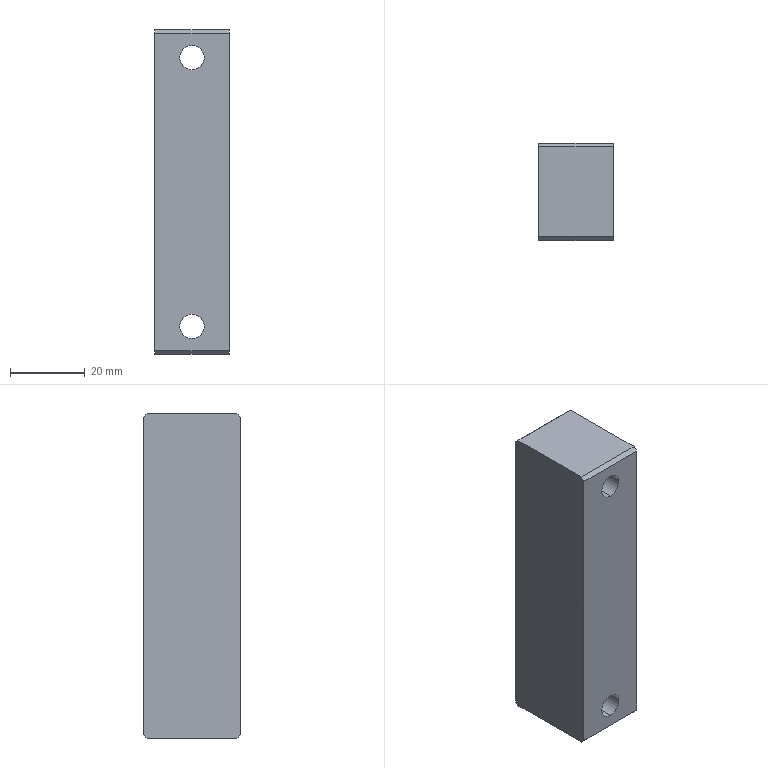Part | STEP file | Riser plate 4_sand-blasted, oxidised | 1 solid | 14 faces | box 20 x 26 x 87 mm | volume 43474 mm3 | plane 10 | cylinder 4 | commonest cylinder face diameters 6.5 x4
STEP:
#1=CARTESIAN_POINT('',(0.,0.,0.));
#2=DIRECTION('',(0.,0.,1.));
#3=DIRECTION('',(1.,0.,0.));
#4=AXIS2_PLACEMENT_3D('',#1,#2,#3);
#5=CARTESIAN_POINT('',(-10.,-13.65,-32.75));
#6=VERTEX_POINT('',#5);
#7=CARTESIAN_POINT('',(-10.,12.35,-32.75));
#8=VERTEX_POINT('',#7);
#9=CARTESIAN_POINT('',(-10.,97.,-32.75));
#10=DIRECTION('',(0.,1.,0.));
#11=VECTOR('',#10,1.);
#12=LINE('',#9,#11);
#13=CARTESIAN_POINT('',(-10.,97.,-36.));
#14=DIRECTION('',(0.,1.,0.));
#15=DIRECTION('',(0.,0.,1.));
#16=AXIS2_PLACEMENT_3D('',#13,#14,#15);
#17=CYLINDRICAL_SURFACE('',#16,3.25);
#18=CARTESIAN_POINT('',(6.283,0.));
#19=DIRECTION('',(0.,1.));
#20=VECTOR('',#19,1.);
#21=LINE('',#18,#20);
#22=(GEOMETRIC_REPRESENTATION_CONTEXT(2)PARAMETRIC_REPRESENTATION_CONTEXT()REPRESENTATION_CONTEXT('',''));
#23=DEFINITIONAL_REPRESENTATION('',(#21),#22);
#24=PCURVE('',#17,#23);
#25=CARTESIAN_POINT('',(-10.,97.,-36.));
#26=DIRECTION('',(0.,1.,0.));
#27=DIRECTION('',(0.,0.,1.));
#28=AXIS2_PLACEMENT_3D('',#25,#26,#27);
#29=CYLINDRICAL_SURFACE('',#28,3.25);
#30=CARTESIAN_POINT('',(0.,0.));
#31=DIRECTION('',(0.,1.));
#32=VECTOR('',#31,1.);
#33=LINE('',#30,#32);
#34=(GEOMETRIC_REPRESENTATION_CONTEXT(2)PARAMETRIC_REPRESENTATION_CONTEXT()REPRESENTATION_CONTEXT('',''));
#35=DEFINITIONAL_REPRESENTATION('',(#33),#34);
#36=PCURVE('',#29,#35);
#37=SURFACE_CURVE('',#12,(#24,#36),.PCURVE_S1.);
#38=EDGE_CURVE('',#6,#8,#37,.T.);
#39=ORIENTED_EDGE('',*,*,#38,.T.);
#40=CARTESIAN_POINT('',(-10.,12.35,-39.25));
#41=VERTEX_POINT('',#40);
#42=CARTESIAN_POINT('',(-10.,12.35,-36.));
#43=DIRECTION('',(0.,-1.,0.));
#44=DIRECTION('',(0.,0.,-1.));
#45=AXIS2_PLACEMENT_3D('',#42,#43,#44);
#46=CIRCLE('',#45,3.25);
#47=CARTESIAN_POINT('',(9.425,-84.65));
#48=DIRECTION('',(-1.,0.));
#49=VECTOR('',#48,1.);
#50=LINE('',#47,#49);
#51=(GEOMETRIC_REPRESENTATION_CONTEXT(2)PARAMETRIC_REPRESENTATION_CONTEXT()REPRESENTATION_CONTEXT('',''));
#52=DEFINITIONAL_REPRESENTATION('',(#50),#51);
#53=PCURVE('',#17,#52);
#54=CARTESIAN_POINT('',(0.,12.35,-43.5));
#55=DIRECTION('',(0.,-1.,0.));
#56=DIRECTION('',(0.,0.,-1.));
#57=AXIS2_PLACEMENT_3D('',#54,#55,#56);
#58=PLANE('',#57);
#59=CARTESIAN_POINT('',(-7.5,-10.));
#60=DIRECTION('',(1.,0.));
#61=AXIS2_PLACEMENT_2D('',#59,#60);
#62=CIRCLE('',#61,3.25);
#63=(GEOMETRIC_REPRESENTATION_CONTEXT(2)PARAMETRIC_REPRESENTATION_CONTEXT()REPRESENTATION_CONTEXT('',''));
#64=DEFINITIONAL_REPRESENTATION('',(#62),#63);
#65=PCURVE('',#58,#64);
#66=SURFACE_CURVE('',#46,(#53,#65),.PCURVE_S1.);
#67=EDGE_CURVE('',#8,#41,#66,.T.);
#68=ORIENTED_EDGE('',*,*,#67,.T.);
#69=CARTESIAN_POINT('',(-10.,-13.65,-39.25));
#70=VERTEX_POINT('',#69);
#71=CARTESIAN_POINT('',(-10.,97.,-39.25));
#72=DIRECTION('',(0.,1.,0.));
#73=VECTOR('',#72,1.);
#74=LINE('',#71,#73);
#75=CARTESIAN_POINT('',(3.142,0.));
#76=DIRECTION('',(0.,1.));
#77=VECTOR('',#76,1.);
#78=LINE('',#75,#77);
#79=(GEOMETRIC_REPRESENTATION_CONTEXT(2)PARAMETRIC_REPRESENTATION_CONTEXT()REPRESENTATION_CONTEXT('',''));
#80=DEFINITIONAL_REPRESENTATION('',(#78),#79);
#81=PCURVE('',#17,#80);
#82=CARTESIAN_POINT('',(3.142,0.));
#83=DIRECTION('',(0.,1.));
#84=VECTOR('',#83,1.);
#85=LINE('',#82,#84);
#86=(GEOMETRIC_REPRESENTATION_CONTEXT(2)PARAMETRIC_REPRESENTATION_CONTEXT()REPRESENTATION_CONTEXT('',''));
#87=DEFINITIONAL_REPRESENTATION('',(#85),#86);
#88=PCURVE('',#29,#87);
#89=SURFACE_CURVE('',#74,(#81,#88),.PCURVE_S1.);
#90=EDGE_CURVE('',#70,#41,#89,.T.);
#91=ORIENTED_EDGE('',*,*,#90,.F.);
#92=CARTESIAN_POINT('',(-10.,-13.65,-36.));
#93=DIRECTION('',(0.,1.,0.));
#94=DIRECTION('',(0.,0.,1.));
#95=AXIS2_PLACEMENT_3D('',#92,#93,#94);
#96=CIRCLE('',#95,3.25);
#97=CARTESIAN_POINT('',(0.,-110.65));
#98=DIRECTION('',(1.,0.));
#99=VECTOR('',#98,1.);
#100=LINE('',#97,#99);
#101=(GEOMETRIC_REPRESENTATION_CONTEXT(2)PARAMETRIC_REPRESENTATION_CONTEXT()REPRESENTATION_CONTEXT('',''));
#102=DEFINITIONAL_REPRESENTATION('',(#100),#101);
#103=PCURVE('',#17,#102);
#104=CARTESIAN_POINT('',(0.,-13.65,43.5));
#105=DIRECTION('',(0.,1.,0.));
#106=DIRECTION('',(-1.,0.,0.));
#107=AXIS2_PLACEMENT_3D('',#104,#105,#106);
#108=PLANE('',#107);
#109=CARTESIAN_POINT('',(10.,-79.5));
#110=DIRECTION('',(0.,1.));
#111=AXIS2_PLACEMENT_2D('',#109,#110);
#112=CIRCLE('',#111,3.25);
#113=(GEOMETRIC_REPRESENTATION_CONTEXT(2)PARAMETRIC_REPRESENTATION_CONTEXT()REPRESENTATION_CONTEXT('',''));
#114=DEFINITIONAL_REPRESENTATION('',(#112),#113);
#115=PCURVE('',#108,#114);
#116=SURFACE_CURVE('',#96,(#103,#115),.PCURVE_S1.);
#117=EDGE_CURVE('',#70,#6,#116,.T.);
#118=ORIENTED_EDGE('',*,*,#117,.T.);
#119=EDGE_LOOP('',(#39,#68,#91,#118));
#120=FACE_BOUND('',#119,.F.);
#121=ADVANCED_FACE('',(#120),#17,.F.);
#122=CARTESIAN_POINT('',(-10.,-13.65,39.25));
#123=VERTEX_POINT('',#122);
#124=CARTESIAN_POINT('',(-10.,12.35,39.25));
#125=VERTEX_POINT('',#124);
#126=CARTESIAN_POINT('',(-10.,97.,39.25));
#127=DIRECTION('',(0.,1.,0.));
#128=VECTOR('',#127,1.);
#129=LINE('',#126,#128);
#130=CARTESIAN_POINT('',(-10.,97.,36.));
#131=DIRECTION('',(0.,1.,0.));
#132=DIRECTION('',(0.,0.,1.));
#133=AXIS2_PLACEMENT_3D('',#130,#131,#132);
#134=CYLINDRICAL_SURFACE('',#133,3.25);
#135=CARTESIAN_POINT('',(6.283,0.));
#136=DIRECTION('',(0.,1.));
#137=VECTOR('',#136,1.);
#138=LINE('',#135,#137);
#139=(GEOMETRIC_REPRESENTATION_CONTEXT(2)PARAMETRIC_REPRESENTATION_CONTEXT()REPRESENTATION_CONTEXT('',''));
#140=DEFINITIONAL_REPRESENTATION('',(#138),#139);
#141=PCURVE('',#134,#140);
#142=CARTESIAN_POINT('',(-10.,97.,36.));
#143=DIRECTION('',(0.,1.,0.));
#144=DIRECTION('',(0.,0.,1.));
#145=AXIS2_PLACEMENT_3D('',#142,#143,#144);
#146=CYLINDRICAL_SURFACE('',#145,3.25);
#147=CARTESIAN_POINT('',(0.,0.));
#148=DIRECTION('',(0.,1.));
#149=VECTOR('',#148,1.);
#150=LINE('',#147,#149);
#151=(GEOMETRIC_REPRESENTATION_CONTEXT(2)PARAMETRIC_REPRESENTATION_CONTEXT()REPRESENTATION_CONTEXT('',''));
#152=DEFINITIONAL_REPRESENTATION('',(#150),#151);
#153=PCURVE('',#146,#152);
#154=SURFACE_CURVE('',#129,(#141,#153),.PCURVE_S1.);
#155=EDGE_CURVE('',#123,#125,#154,.T.);
#156=ORIENTED_EDGE('',*,*,#155,.T.);
#157=CARTESIAN_POINT('',(-10.,12.35,32.75));
#158=VERTEX_POINT('',#157);
#159=CARTESIAN_POINT('',(-10.,12.35,36.));
#160=DIRECTION('',(0.,-1.,0.));
#161=DIRECTION('',(0.,0.,-1.));
#162=AXIS2_PLACEMENT_3D('',#159,#160,#161);
#163=CIRCLE('',#162,3.25);
#164=CARTESIAN_POINT('',(9.425,-84.65));
#165=DIRECTION('',(-1.,0.));
#166=VECTOR('',#165,1.);
#167=LINE('',#164,#166);
#168=(GEOMETRIC_REPRESENTATION_CONTEXT(2)PARAMETRIC_REPRESENTATION_CONTEXT()REPRESENTATION_CONTEXT('',''));
#169=DEFINITIONAL_REPRESENTATION('',(#167),#168);
#170=PCURVE('',#134,#169);
#171=CARTESIAN_POINT('',(-79.5,-10.));
#172=DIRECTION('',(1.,0.));
#173=AXIS2_PLACEMENT_2D('',#171,#172);
#174=CIRCLE('',#173,3.25);
#175=(GEOMETRIC_REPRESENTATION_CONTEXT(2)PARAMETRIC_REPRESENTATION_CONTEXT()REPRESENTATION_CONTEXT('',''));
#176=DEFINITIONAL_REPRESENTATION('',(#174),#175);
#177=PCURVE('',#58,#176);
#178=SURFACE_CURVE('',#163,(#170,#177),.PCURVE_S1.);
#179=EDGE_CURVE('',#125,#158,#178,.T.);
#180=ORIENTED_EDGE('',*,*,#179,.T.);
#181=CARTESIAN_POINT('',(-10.,-13.65,32.75));
#182=VERTEX_POINT('',#181);
#183=CARTESIAN_POINT('',(-10.,97.,32.75));
#184=DIRECTION('',(0.,1.,0.));
#185=VECTOR('',#184,1.);
#186=LINE('',#183,#185);
#187=CARTESIAN_POINT('',(3.142,0.));
#188=DIRECTION('',(0.,1.));
#189=VECTOR('',#188,1.);
#190=LINE('',#187,#189);
#191=(GEOMETRIC_REPRESENTATION_CONTEXT(2)PARAMETRIC_REPRESENTATION_CONTEXT()REPRESENTATION_CONTEXT('',''));
#192=DEFINITIONAL_REPRESENTATION('',(#190),#191);
#193=PCURVE('',#134,#192);
#194=CARTESIAN_POINT('',(3.142,0.));
#195=DIRECTION('',(0.,1.));
#196=VECTOR('',#195,1.);
#197=LINE('',#194,#196);
#198=(GEOMETRIC_REPRESENTATION_CONTEXT(2)PARAMETRIC_REPRESENTATION_CONTEXT()REPRESENTATION_CONTEXT('',''));
#199=DEFINITIONAL_REPRESENTATION('',(#197),#198);
#200=PCURVE('',#146,#199);
#201=SURFACE_CURVE('',#186,(#193,#200),.PCURVE_S1.);
#202=EDGE_CURVE('',#182,#158,#201,.T.);
#203=ORIENTED_EDGE('',*,*,#202,.F.);
#204=CARTESIAN_POINT('',(-10.,-13.65,36.));
#205=DIRECTION('',(0.,1.,0.));
#206=DIRECTION('',(0.,0.,1.));
#207=AXIS2_PLACEMENT_3D('',#204,#205,#206);
#208=CIRCLE('',#207,3.25);
#209=CARTESIAN_POINT('',(0.,-110.65));
#210=DIRECTION('',(1.,0.));
#211=VECTOR('',#210,1.);
#212=LINE('',#209,#211);
#213=(GEOMETRIC_REPRESENTATION_CONTEXT(2)PARAMETRIC_REPRESENTATION_CONTEXT()REPRESENTATION_CONTEXT('',''));
#214=DEFINITIONAL_REPRESENTATION('',(#212),#213);
#215=PCURVE('',#134,#214);
#216=CARTESIAN_POINT('',(10.,-7.5));
#217=DIRECTION('',(0.,1.));
#218=AXIS2_PLACEMENT_2D('',#216,#217);
#219=CIRCLE('',#218,3.25);
#220=(GEOMETRIC_REPRESENTATION_CONTEXT(2)PARAMETRIC_REPRESENTATION_CONTEXT()REPRESENTATION_CONTEXT('',''));
#221=DEFINITIONAL_REPRESENTATION('',(#219),#220);
#222=PCURVE('',#108,#221);
#223=SURFACE_CURVE('',#208,(#215,#222),.PCURVE_S1.);
#224=EDGE_CURVE('',#182,#123,#223,.T.);
#225=ORIENTED_EDGE('',*,*,#224,.T.);
#226=EDGE_LOOP('',(#156,#180,#203,#225));
#227=FACE_BOUND('',#226,.F.);
#228=ADVANCED_FACE('',(#227),#134,.F.);
#229=CARTESIAN_POINT('',(-20.,11.35,43.5));
#230=VERTEX_POINT('',#229);
#231=CARTESIAN_POINT('',(-20.,-12.65,43.5));
#232=VERTEX_POINT('',#231);
#233=CARTESIAN_POINT('',(-20.,0.,43.5));
#234=DIRECTION('',(0.,-1.,0.));
#235=VECTOR('',#234,1.);
#236=LINE('',#233,#235);
#237=CARTESIAN_POINT('',(0.,0.,43.5));
#238=DIRECTION('',(0.,0.,-1.));
#239=DIRECTION('',(-1.,0.,0.));
#240=AXIS2_PLACEMENT_3D('',#237,#238,#239);
#241=PLANE('',#240);
#242=CARTESIAN_POINT('',(20.,0.));
#243=DIRECTION('',(0.,-1.));
#244=VECTOR('',#243,1.);
#245=LINE('',#242,#244);
#246=(GEOMETRIC_REPRESENTATION_CONTEXT(2)PARAMETRIC_REPRESENTATION_CONTEXT()REPRESENTATION_CONTEXT('',''));
#247=DEFINITIONAL_REPRESENTATION('',(#245),#246);
#248=PCURVE('',#241,#247);
#249=CARTESIAN_POINT('',(-20.,0.,43.5));
#250=DIRECTION('',(1.,0.,0.));
#251=DIRECTION('',(0.,0.,-1.));
#252=AXIS2_PLACEMENT_3D('',#249,#250,#251);
#253=PLANE('',#252);
#254=CARTESIAN_POINT('',(0.,0.));
#255=DIRECTION('',(0.,-1.));
#256=VECTOR('',#255,1.);
#257=LINE('',#254,#256);
#258=(GEOMETRIC_REPRESENTATION_CONTEXT(2)PARAMETRIC_REPRESENTATION_CONTEXT()REPRESENTATION_CONTEXT('',''));
#259=DEFINITIONAL_REPRESENTATION('',(#257),#258);
#260=PCURVE('',#253,#259);
#261=SURFACE_CURVE('',#236,(#248,#260),.PCURVE_S1.);
#262=EDGE_CURVE('',#230,#232,#261,.T.);
#263=ORIENTED_EDGE('',*,*,#262,.T.);
#264=CARTESIAN_POINT('',(0.,-12.65,43.5));
#265=VERTEX_POINT('',#264);
#266=CARTESIAN_POINT('',(0.,-12.65,43.5));
#267=DIRECTION('',(1.,0.,0.));
#268=VECTOR('',#267,1.);
#269=LINE('',#266,#268);
#270=CARTESIAN_POINT('',(0.,-12.65));
#271=DIRECTION('',(-1.,0.));
#272=VECTOR('',#271,1.);
#273=LINE('',#270,#272);
#274=(GEOMETRIC_REPRESENTATION_CONTEXT(2)PARAMETRIC_REPRESENTATION_CONTEXT()REPRESENTATION_CONTEXT('',''));
#275=DEFINITIONAL_REPRESENTATION('',(#273),#274);
#276=PCURVE('',#241,#275);
#277=CARTESIAN_POINT('',(0.,-12.65,43.5));
#278=DIRECTION('',(0.,0.7071,-0.7071));
#279=DIRECTION('',(1.,0.,0.));
#280=AXIS2_PLACEMENT_3D('',#277,#278,#279);
#281=PLANE('',#280);
#282=CARTESIAN_POINT('',(0.,0.));
#283=DIRECTION('',(1.,0.));
#284=VECTOR('',#283,1.);
#285=LINE('',#282,#284);
#286=(GEOMETRIC_REPRESENTATION_CONTEXT(2)PARAMETRIC_REPRESENTATION_CONTEXT()REPRESENTATION_CONTEXT('',''));
#287=DEFINITIONAL_REPRESENTATION('',(#285),#286);
#288=PCURVE('',#281,#287);
#289=SURFACE_CURVE('',#269,(#276,#288),.PCURVE_S1.);
#290=EDGE_CURVE('',#232,#265,#289,.T.);
#291=ORIENTED_EDGE('',*,*,#290,.T.);
#292=CARTESIAN_POINT('',(0.,11.35,43.5));
#293=VERTEX_POINT('',#292);
#294=CARTESIAN_POINT('',(0.,97.,43.5));
#295=DIRECTION('',(0.,1.,0.));
#296=VECTOR('',#295,1.);
#297=LINE('',#294,#296);
#298=CARTESIAN_POINT('',(0.,97.));
#299=DIRECTION('',(0.,1.));
#300=VECTOR('',#299,1.);
#301=LINE('',#298,#300);
#302=(GEOMETRIC_REPRESENTATION_CONTEXT(2)PARAMETRIC_REPRESENTATION_CONTEXT()REPRESENTATION_CONTEXT('',''));
#303=DEFINITIONAL_REPRESENTATION('',(#301),#302);
#304=PCURVE('',#241,#303);
#305=CARTESIAN_POINT('',(0.,97.,43.5));
#306=DIRECTION('',(-1.,0.,0.));
#307=DIRECTION('',(0.,-1.,0.));
#308=AXIS2_PLACEMENT_3D('',#305,#306,#307);
#309=PLANE('',#308);
#310=CARTESIAN_POINT('',(0.,0.));
#311=DIRECTION('',(-1.,0.));
#312=VECTOR('',#311,1.);
#313=LINE('',#310,#312);
#314=(GEOMETRIC_REPRESENTATION_CONTEXT(2)PARAMETRIC_REPRESENTATION_CONTEXT()REPRESENTATION_CONTEXT('',''));
#315=DEFINITIONAL_REPRESENTATION('',(#313),#314);
#316=PCURVE('',#309,#315);
#317=SURFACE_CURVE('',#297,(#304,#316),.PCURVE_S1.);
#318=EDGE_CURVE('',#265,#293,#317,.T.);
#319=ORIENTED_EDGE('',*,*,#318,.T.);
#320=CARTESIAN_POINT('',(0.,11.35,43.5));
#321=DIRECTION('',(-1.,0.,0.));
#322=VECTOR('',#321,1.);
#323=LINE('',#320,#322);
#324=CARTESIAN_POINT('',(0.,11.35));
#325=DIRECTION('',(1.,0.));
#326=VECTOR('',#325,1.);
#327=LINE('',#324,#326);
#328=(GEOMETRIC_REPRESENTATION_CONTEXT(2)PARAMETRIC_REPRESENTATION_CONTEXT()REPRESENTATION_CONTEXT('',''));
#329=DEFINITIONAL_REPRESENTATION('',(#327),#328);
#330=PCURVE('',#241,#329);
#331=CARTESIAN_POINT('',(0.,11.35,43.5));
#332=DIRECTION('',(0.,-0.7071,-0.7071));
#333=DIRECTION('',(-1.,0.,0.));
#334=AXIS2_PLACEMENT_3D('',#331,#332,#333);
#335=PLANE('',#334);
#336=CARTESIAN_POINT('',(0.,0.));
#337=DIRECTION('',(1.,0.));
#338=VECTOR('',#337,1.);
#339=LINE('',#336,#338);
#340=(GEOMETRIC_REPRESENTATION_CONTEXT(2)PARAMETRIC_REPRESENTATION_CONTEXT()REPRESENTATION_CONTEXT('',''));
#341=DEFINITIONAL_REPRESENTATION('',(#339),#340);
#342=PCURVE('',#335,#341);
#343=SURFACE_CURVE('',#323,(#330,#342),.PCURVE_S1.);
#344=EDGE_CURVE('',#293,#230,#343,.T.);
#345=ORIENTED_EDGE('',*,*,#344,.T.);
#346=EDGE_LOOP('',(#263,#291,#319,#345));
#347=FACE_BOUND('',#346,.T.);
#348=ADVANCED_FACE('',(#347),#241,.F.);
#349=CARTESIAN_POINT('',(0.,11.35,-43.5));
#350=VERTEX_POINT('',#349);
#351=CARTESIAN_POINT('',(0.,12.35,-42.5));
#352=VERTEX_POINT('',#351);
#353=CARTESIAN_POINT('',(0.,12.35,-42.5));
#354=DIRECTION('',(0.,0.7071,0.7071));
#355=VECTOR('',#354,1.);
#356=LINE('',#353,#355);
#357=CARTESIAN_POINT('',(84.65,-86.));
#358=DIRECTION('',(-0.7071,0.7071));
#359=VECTOR('',#358,1.);
#360=LINE('',#357,#359);
#361=(GEOMETRIC_REPRESENTATION_CONTEXT(2)PARAMETRIC_REPRESENTATION_CONTEXT()REPRESENTATION_CONTEXT('',''));
#362=DEFINITIONAL_REPRESENTATION('',(#360),#361);
#363=PCURVE('',#309,#362);
#364=CARTESIAN_POINT('',(0.,12.35,-42.5));
#365=DIRECTION('',(0.,0.7071,-0.7071));
#366=DIRECTION('',(1.,0.,0.));
#367=AXIS2_PLACEMENT_3D('',#364,#365,#366);
#368=PLANE('',#367);
#369=CARTESIAN_POINT('',(0.,0.));
#370=DIRECTION('',(0.,-1.));
#371=VECTOR('',#370,1.);
#372=LINE('',#369,#371);
#373=(GEOMETRIC_REPRESENTATION_CONTEXT(2)PARAMETRIC_REPRESENTATION_CONTEXT()REPRESENTATION_CONTEXT('',''));
#374=DEFINITIONAL_REPRESENTATION('',(#372),#373);
#375=PCURVE('',#368,#374);
#376=SURFACE_CURVE('',#356,(#363,#375),.PCURVE_S1.);
#377=EDGE_CURVE('',#350,#352,#376,.T.);
#378=ORIENTED_EDGE('',*,*,#377,.T.);
#379=CARTESIAN_POINT('',(0.,12.35,42.5));
#380=VERTEX_POINT('',#379);
#381=CARTESIAN_POINT('',(0.,12.35,43.5));
#382=DIRECTION('',(0.,0.,1.));
#383=VECTOR('',#382,1.);
#384=LINE('',#381,#383);
#385=CARTESIAN_POINT('',(84.65,0.));
#386=DIRECTION('',(0.,1.));
#387=VECTOR('',#386,1.);
#388=LINE('',#385,#387);
#389=(GEOMETRIC_REPRESENTATION_CONTEXT(2)PARAMETRIC_REPRESENTATION_CONTEXT()REPRESENTATION_CONTEXT('',''));
#390=DEFINITIONAL_REPRESENTATION('',(#388),#389);
#391=PCURVE('',#309,#390);
#392=CARTESIAN_POINT('',(-87.,0.));
#393=DIRECTION('',(-1.,0.));
#394=VECTOR('',#393,1.);
#395=LINE('',#392,#394);
#396=(GEOMETRIC_REPRESENTATION_CONTEXT(2)PARAMETRIC_REPRESENTATION_CONTEXT()REPRESENTATION_CONTEXT('',''));
#397=DEFINITIONAL_REPRESENTATION('',(#395),#396);
#398=PCURVE('',#58,#397);
#399=SURFACE_CURVE('',#384,(#391,#398),.PCURVE_S1.);
#400=EDGE_CURVE('',#352,#380,#399,.T.);
#401=ORIENTED_EDGE('',*,*,#400,.T.);
#402=CARTESIAN_POINT('',(0.,11.35,43.5));
#403=DIRECTION('',(0.,-0.7071,0.7071));
#404=VECTOR('',#403,1.);
#405=LINE('',#402,#404);
#406=CARTESIAN_POINT('',(85.65,0.));
#407=DIRECTION('',(0.7071,0.7071));
#408=VECTOR('',#407,1.);
#409=LINE('',#406,#408);
#410=(GEOMETRIC_REPRESENTATION_CONTEXT(2)PARAMETRIC_REPRESENTATION_CONTEXT()REPRESENTATION_CONTEXT('',''));
#411=DEFINITIONAL_REPRESENTATION('',(#409),#410);
#412=PCURVE('',#309,#411);
#413=CARTESIAN_POINT('',(0.,0.));
#414=DIRECTION('',(0.,-1.));
#415=VECTOR('',#414,1.);
#416=LINE('',#413,#415);
#417=(GEOMETRIC_REPRESENTATION_CONTEXT(2)PARAMETRIC_REPRESENTATION_CONTEXT()REPRESENTATION_CONTEXT('',''));
#418=DEFINITIONAL_REPRESENTATION('',(#416),#417);
#419=PCURVE('',#335,#418);
#420=SURFACE_CURVE('',#405,(#412,#419),.PCURVE_S1.);
#421=EDGE_CURVE('',#380,#293,#420,.T.);
#422=ORIENTED_EDGE('',*,*,#421,.T.);
#423=ORIENTED_EDGE('',*,*,#318,.F.);
#424=CARTESIAN_POINT('',(0.,-13.65,42.5));
#425=VERTEX_POINT('',#424);
#426=CARTESIAN_POINT('',(0.,-12.65,43.5));
#427=DIRECTION('',(0.,-0.7071,-0.7071));
#428=VECTOR('',#427,1.);
#429=LINE('',#426,#428);
#430=CARTESIAN_POINT('',(109.65,0.));
#431=DIRECTION('',(0.7071,-0.7071));
#432=VECTOR('',#431,1.);
#433=LINE('',#430,#432);
#434=(GEOMETRIC_REPRESENTATION_CONTEXT(2)PARAMETRIC_REPRESENTATION_CONTEXT()REPRESENTATION_CONTEXT('',''));
#435=DEFINITIONAL_REPRESENTATION('',(#433),#434);
#436=PCURVE('',#309,#435);
#437=CARTESIAN_POINT('',(0.,0.));
#438=DIRECTION('',(0.,1.));
#439=VECTOR('',#438,1.);
#440=LINE('',#437,#439);
#441=(GEOMETRIC_REPRESENTATION_CONTEXT(2)PARAMETRIC_REPRESENTATION_CONTEXT()REPRESENTATION_CONTEXT('',''));
#442=DEFINITIONAL_REPRESENTATION('',(#440),#441);
#443=PCURVE('',#281,#442);
#444=SURFACE_CURVE('',#429,(#436,#443),.PCURVE_S1.);
#445=EDGE_CURVE('',#265,#425,#444,.T.);
#446=ORIENTED_EDGE('',*,*,#445,.T.);
#447=CARTESIAN_POINT('',(0.,-13.65,-42.5));
#448=VERTEX_POINT('',#447);
#449=CARTESIAN_POINT('',(0.,-13.65,43.5));
#450=DIRECTION('',(0.,0.,-1.));
#451=VECTOR('',#450,1.);
#452=LINE('',#449,#451);
#453=CARTESIAN_POINT('',(110.65,0.));
#454=DIRECTION('',(0.,-1.));
#455=VECTOR('',#454,1.);
#456=LINE('',#453,#455);
#457=(GEOMETRIC_REPRESENTATION_CONTEXT(2)PARAMETRIC_REPRESENTATION_CONTEXT()REPRESENTATION_CONTEXT('',''));
#458=DEFINITIONAL_REPRESENTATION('',(#456),#457);
#459=PCURVE('',#309,#458);
#460=CARTESIAN_POINT('',(0.,0.));
#461=DIRECTION('',(0.,-1.));
#462=VECTOR('',#461,1.);
#463=LINE('',#460,#462);
#464=(GEOMETRIC_REPRESENTATION_CONTEXT(2)PARAMETRIC_REPRESENTATION_CONTEXT()REPRESENTATION_CONTEXT('',''));
#465=DEFINITIONAL_REPRESENTATION('',(#463),#464);
#466=PCURVE('',#108,#465);
#467=SURFACE_CURVE('',#452,(#459,#466),.PCURVE_S1.);
#468=EDGE_CURVE('',#425,#448,#467,.T.);
#469=ORIENTED_EDGE('',*,*,#468,.T.);
#470=CARTESIAN_POINT('',(0.,-12.65,-43.5));
#471=VERTEX_POINT('',#470);
#472=CARTESIAN_POINT('',(0.,-13.65,-42.5));
#473=DIRECTION('',(0.,0.7071,-0.7071));
#474=VECTOR('',#473,1.);
#475=LINE('',#472,#474);
#476=CARTESIAN_POINT('',(110.65,-86.));
#477=DIRECTION('',(-0.7071,-0.7071));
#478=VECTOR('',#477,1.);
#479=LINE('',#476,#478);
#480=(GEOMETRIC_REPRESENTATION_CONTEXT(2)PARAMETRIC_REPRESENTATION_CONTEXT()REPRESENTATION_CONTEXT('',''));
#481=DEFINITIONAL_REPRESENTATION('',(#479),#480);
#482=PCURVE('',#309,#481);
#483=CARTESIAN_POINT('',(0.,-13.65,-42.5));
#484=DIRECTION('',(0.,-0.7071,-0.7071));
#485=DIRECTION('',(-1.,0.,0.));
#486=AXIS2_PLACEMENT_3D('',#483,#484,#485);
#487=PLANE('',#486);
#488=CARTESIAN_POINT('',(0.,0.));
#489=DIRECTION('',(0.,1.));
#490=VECTOR('',#489,1.);
#491=LINE('',#488,#490);
#492=(GEOMETRIC_REPRESENTATION_CONTEXT(2)PARAMETRIC_REPRESENTATION_CONTEXT()REPRESENTATION_CONTEXT('',''));
#493=DEFINITIONAL_REPRESENTATION('',(#491),#492);
#494=PCURVE('',#487,#493);
#495=SURFACE_CURVE('',#475,(#482,#494),.PCURVE_S1.);
#496=EDGE_CURVE('',#448,#471,#495,.T.);
#497=ORIENTED_EDGE('',*,*,#496,.T.);
#498=CARTESIAN_POINT('',(0.,97.,-43.5));
#499=DIRECTION('',(0.,1.,0.));
#500=VECTOR('',#499,1.);
#501=LINE('',#498,#500);
#502=CARTESIAN_POINT('',(0.,-87.));
#503=DIRECTION('',(-1.,0.));
#504=VECTOR('',#503,1.);
#505=LINE('',#502,#504);
#506=(GEOMETRIC_REPRESENTATION_CONTEXT(2)PARAMETRIC_REPRESENTATION_CONTEXT()REPRESENTATION_CONTEXT('',''));
#507=DEFINITIONAL_REPRESENTATION('',(#505),#506);
#508=PCURVE('',#309,#507);
#509=CARTESIAN_POINT('',(0.,0.,-43.5));
#510=DIRECTION('',(0.,0.,-1.));
#511=DIRECTION('',(-1.,0.,0.));
#512=AXIS2_PLACEMENT_3D('',#509,#510,#511);
#513=PLANE('',#512);
#514=CARTESIAN_POINT('',(0.,97.));
#515=DIRECTION('',(0.,1.));
#516=VECTOR('',#515,1.);
#517=LINE('',#514,#516);
#518=(GEOMETRIC_REPRESENTATION_CONTEXT(2)PARAMETRIC_REPRESENTATION_CONTEXT()REPRESENTATION_CONTEXT('',''));
#519=DEFINITIONAL_REPRESENTATION('',(#517),#518);
#520=PCURVE('',#513,#519);
#521=SURFACE_CURVE('',#501,(#508,#520),.PCURVE_S1.);
#522=EDGE_CURVE('',#471,#350,#521,.T.);
#523=ORIENTED_EDGE('',*,*,#522,.T.);
#524=EDGE_LOOP('',(#378,#401,#422,#423,#446,#469,#497,#523));
#525=FACE_BOUND('',#524,.T.);
#526=ADVANCED_FACE('',(#525),#309,.F.);
#527=CARTESIAN_POINT('',(-20.,12.35,-42.5));
#528=VERTEX_POINT('',#527);
#529=CARTESIAN_POINT('',(-20.,12.35,42.5));
#530=VERTEX_POINT('',#529);
#531=CARTESIAN_POINT('',(-20.,12.35,43.5));
#532=DIRECTION('',(0.,0.,1.));
#533=VECTOR('',#532,1.);
#534=LINE('',#531,#533);
#535=CARTESIAN_POINT('',(0.,12.35));
#536=DIRECTION('',(-1.,0.));
#537=VECTOR('',#536,1.);
#538=LINE('',#535,#537);
#539=(GEOMETRIC_REPRESENTATION_CONTEXT(2)PARAMETRIC_REPRESENTATION_CONTEXT()REPRESENTATION_CONTEXT('',''));
#540=DEFINITIONAL_REPRESENTATION('',(#538),#539);
#541=PCURVE('',#253,#540);
#542=CARTESIAN_POINT('',(-87.,-20.));
#543=DIRECTION('',(-1.,0.));
#544=VECTOR('',#543,1.);
#545=LINE('',#542,#544);
#546=(GEOMETRIC_REPRESENTATION_CONTEXT(2)PARAMETRIC_REPRESENTATION_CONTEXT()REPRESENTATION_CONTEXT('',''));
#547=DEFINITIONAL_REPRESENTATION('',(#545),#546);
#548=PCURVE('',#58,#547);
#549=SURFACE_CURVE('',#534,(#541,#548),.PCURVE_S1.);
#550=EDGE_CURVE('',#528,#530,#549,.T.);
#551=ORIENTED_EDGE('',*,*,#550,.F.);
#552=CARTESIAN_POINT('',(-20.,11.35,-43.5));
#553=VERTEX_POINT('',#552);
#554=CARTESIAN_POINT('',(-20.,12.35,-42.5));
#555=DIRECTION('',(0.,-0.7071,-0.7071));
#556=VECTOR('',#555,1.);
#557=LINE('',#554,#556);
#558=CARTESIAN_POINT('',(86.,12.35));
#559=DIRECTION('',(0.7071,-0.7071));
#560=VECTOR('',#559,1.);
#561=LINE('',#558,#560);
#562=(GEOMETRIC_REPRESENTATION_CONTEXT(2)PARAMETRIC_REPRESENTATION_CONTEXT()REPRESENTATION_CONTEXT('',''));
#563=DEFINITIONAL_REPRESENTATION('',(#561),#562);
#564=PCURVE('',#253,#563);
#565=CARTESIAN_POINT('',(-20.,0.));
#566=DIRECTION('',(0.,1.));
#567=VECTOR('',#566,1.);
#568=LINE('',#565,#567);
#569=(GEOMETRIC_REPRESENTATION_CONTEXT(2)PARAMETRIC_REPRESENTATION_CONTEXT()REPRESENTATION_CONTEXT('',''));
#570=DEFINITIONAL_REPRESENTATION('',(#568),#569);
#571=PCURVE('',#368,#570);
#572=SURFACE_CURVE('',#557,(#564,#571),.PCURVE_S1.);
#573=EDGE_CURVE('',#528,#553,#572,.T.);
#574=ORIENTED_EDGE('',*,*,#573,.T.);
#575=CARTESIAN_POINT('',(-20.,-12.65,-43.5));
#576=VERTEX_POINT('',#575);
#577=CARTESIAN_POINT('',(-20.,0.,-43.5));
#578=DIRECTION('',(0.,-1.,0.));
#579=VECTOR('',#578,1.);
#580=LINE('',#577,#579);
#581=CARTESIAN_POINT('',(87.,0.));
#582=DIRECTION('',(0.,-1.));
#583=VECTOR('',#582,1.);
#584=LINE('',#581,#583);
#585=(GEOMETRIC_REPRESENTATION_CONTEXT(2)PARAMETRIC_REPRESENTATION_CONTEXT()REPRESENTATION_CONTEXT('',''));
#586=DEFINITIONAL_REPRESENTATION('',(#584),#585);
#587=PCURVE('',#253,#586);
#588=CARTESIAN_POINT('',(20.,0.));
#589=DIRECTION('',(0.,-1.));
#590=VECTOR('',#589,1.);
#591=LINE('',#588,#590);
#592=(GEOMETRIC_REPRESENTATION_CONTEXT(2)PARAMETRIC_REPRESENTATION_CONTEXT()REPRESENTATION_CONTEXT('',''));
#593=DEFINITIONAL_REPRESENTATION('',(#591),#592);
#594=PCURVE('',#513,#593);
#595=SURFACE_CURVE('',#580,(#587,#594),.PCURVE_S1.);
#596=EDGE_CURVE('',#553,#576,#595,.T.);
#597=ORIENTED_EDGE('',*,*,#596,.T.);
#598=CARTESIAN_POINT('',(-20.,-13.65,-42.5));
#599=VERTEX_POINT('',#598);
#600=CARTESIAN_POINT('',(-20.,-13.65,-42.5));
#601=DIRECTION('',(0.,-0.7071,0.7071));
#602=VECTOR('',#601,1.);
#603=LINE('',#600,#602);
#604=CARTESIAN_POINT('',(86.,-13.65));
#605=DIRECTION('',(-0.7071,-0.7071));
#606=VECTOR('',#605,1.);
#607=LINE('',#604,#606);
#608=(GEOMETRIC_REPRESENTATION_CONTEXT(2)PARAMETRIC_REPRESENTATION_CONTEXT()REPRESENTATION_CONTEXT('',''));
#609=DEFINITIONAL_REPRESENTATION('',(#607),#608);
#610=PCURVE('',#253,#609);
#611=CARTESIAN_POINT('',(20.,0.));
#612=DIRECTION('',(0.,-1.));
#613=VECTOR('',#612,1.);
#614=LINE('',#611,#613);
#615=(GEOMETRIC_REPRESENTATION_CONTEXT(2)PARAMETRIC_REPRESENTATION_CONTEXT()REPRESENTATION_CONTEXT('',''));
#616=DEFINITIONAL_REPRESENTATION('',(#614),#615);
#617=PCURVE('',#487,#616);
#618=SURFACE_CURVE('',#603,(#610,#617),.PCURVE_S1.);
#619=EDGE_CURVE('',#576,#599,#618,.T.);
#620=ORIENTED_EDGE('',*,*,#619,.T.);
#621=CARTESIAN_POINT('',(-20.,-13.65,42.5));
#622=VERTEX_POINT('',#621);
#623=CARTESIAN_POINT('',(-20.,-13.65,43.5));
#624=DIRECTION('',(0.,0.,-1.));
#625=VECTOR('',#624,1.);
#626=LINE('',#623,#625);
#627=CARTESIAN_POINT('',(0.,-13.65));
#628=DIRECTION('',(1.,0.));
#629=VECTOR('',#628,1.);
#630=LINE('',#627,#629);
#631=(GEOMETRIC_REPRESENTATION_CONTEXT(2)PARAMETRIC_REPRESENTATION_CONTEXT()REPRESENTATION_CONTEXT('',''));
#632=DEFINITIONAL_REPRESENTATION('',(#630),#631);
#633=PCURVE('',#253,#632);
#634=CARTESIAN_POINT('',(20.,0.));
#635=DIRECTION('',(0.,-1.));
#636=VECTOR('',#635,1.);
#637=LINE('',#634,#636);
#638=(GEOMETRIC_REPRESENTATION_CONTEXT(2)PARAMETRIC_REPRESENTATION_CONTEXT()REPRESENTATION_CONTEXT('',''));
#639=DEFINITIONAL_REPRESENTATION('',(#637),#638);
#640=PCURVE('',#108,#639);
#641=SURFACE_CURVE('',#626,(#633,#640),.PCURVE_S1.);
#642=EDGE_CURVE('',#622,#599,#641,.T.);
#643=ORIENTED_EDGE('',*,*,#642,.F.);
#644=CARTESIAN_POINT('',(-20.,-12.65,43.5));
#645=DIRECTION('',(0.,0.7071,0.7071));
#646=VECTOR('',#645,1.);
#647=LINE('',#644,#646);
#648=CARTESIAN_POINT('',(0.,-12.65));
#649=DIRECTION('',(-0.7071,0.7071));
#650=VECTOR('',#649,1.);
#651=LINE('',#648,#650);
#652=(GEOMETRIC_REPRESENTATION_CONTEXT(2)PARAMETRIC_REPRESENTATION_CONTEXT()REPRESENTATION_CONTEXT('',''));
#653=DEFINITIONAL_REPRESENTATION('',(#651),#652);
#654=PCURVE('',#253,#653);
#655=CARTESIAN_POINT('',(-20.,0.));
#656=DIRECTION('',(0.,-1.));
#657=VECTOR('',#656,1.);
#658=LINE('',#655,#657);
#659=(GEOMETRIC_REPRESENTATION_CONTEXT(2)PARAMETRIC_REPRESENTATION_CONTEXT()REPRESENTATION_CONTEXT('',''));
#660=DEFINITIONAL_REPRESENTATION('',(#658),#659);
#661=PCURVE('',#281,#660);
#662=SURFACE_CURVE('',#647,(#654,#661),.PCURVE_S1.);
#663=EDGE_CURVE('',#622,#232,#662,.T.);
#664=ORIENTED_EDGE('',*,*,#663,.T.);
#665=ORIENTED_EDGE('',*,*,#262,.F.);
#666=CARTESIAN_POINT('',(-20.,11.35,43.5));
#667=DIRECTION('',(0.,0.7071,-0.7071));
#668=VECTOR('',#667,1.);
#669=LINE('',#666,#668);
#670=CARTESIAN_POINT('',(0.,11.35));
#671=DIRECTION('',(0.7071,0.7071));
#672=VECTOR('',#671,1.);
#673=LINE('',#670,#672);
#674=(GEOMETRIC_REPRESENTATION_CONTEXT(2)PARAMETRIC_REPRESENTATION_CONTEXT()REPRESENTATION_CONTEXT('',''));
#675=DEFINITIONAL_REPRESENTATION('',(#673),#674);
#676=PCURVE('',#253,#675);
#677=CARTESIAN_POINT('',(20.,0.));
#678=DIRECTION('',(0.,1.));
#679=VECTOR('',#678,1.);
#680=LINE('',#677,#679);
#681=(GEOMETRIC_REPRESENTATION_CONTEXT(2)PARAMETRIC_REPRESENTATION_CONTEXT()REPRESENTATION_CONTEXT('',''));
#682=DEFINITIONAL_REPRESENTATION('',(#680),#681);
#683=PCURVE('',#335,#682);
#684=SURFACE_CURVE('',#669,(#676,#683),.PCURVE_S1.);
#685=EDGE_CURVE('',#230,#530,#684,.T.);
#686=ORIENTED_EDGE('',*,*,#685,.T.);
#687=EDGE_LOOP('',(#551,#574,#597,#620,#643,#664,#665,#686));
#688=FACE_BOUND('',#687,.T.);
#689=ADVANCED_FACE('',(#688),#253,.F.);
#690=CARTESIAN_POINT('',(-10.,-13.65,-36.));
#691=DIRECTION('',(0.,1.,0.));
#692=DIRECTION('',(0.,0.,1.));
#693=AXIS2_PLACEMENT_3D('',#690,#691,#692);
#694=CIRCLE('',#693,3.25);
#695=CARTESIAN_POINT('',(10.,-79.5));
#696=DIRECTION('',(0.,1.));
#697=AXIS2_PLACEMENT_2D('',#695,#696);
#698=CIRCLE('',#697,3.25);
#699=(GEOMETRIC_REPRESENTATION_CONTEXT(2)PARAMETRIC_REPRESENTATION_CONTEXT()REPRESENTATION_CONTEXT('',''));
#700=DEFINITIONAL_REPRESENTATION('',(#698),#699);
#701=PCURVE('',#108,#700);
#702=CARTESIAN_POINT('',(0.,-110.65));
#703=DIRECTION('',(1.,0.));
#704=VECTOR('',#703,1.);
#705=LINE('',#702,#704);
#706=(GEOMETRIC_REPRESENTATION_CONTEXT(2)PARAMETRIC_REPRESENTATION_CONTEXT()REPRESENTATION_CONTEXT('',''));
#707=DEFINITIONAL_REPRESENTATION('',(#705),#706);
#708=PCURVE('',#29,#707);
#709=SURFACE_CURVE('',#694,(#701,#708),.PCURVE_S1.);
#710=EDGE_CURVE('',#6,#70,#709,.T.);
#711=ORIENTED_EDGE('',*,*,#710,.T.);
#712=ORIENTED_EDGE('',*,*,#117,.T.);
#713=EDGE_LOOP('',(#711,#712));
#714=FACE_BOUND('',#713,.T.);
#715=CARTESIAN_POINT('',(-10.,-13.65,36.));
#716=DIRECTION('',(0.,1.,0.));
#717=DIRECTION('',(0.,0.,1.));
#718=AXIS2_PLACEMENT_3D('',#715,#716,#717);
#719=CIRCLE('',#718,3.25);
#720=CARTESIAN_POINT('',(10.,-7.5));
#721=DIRECTION('',(0.,1.));
#722=AXIS2_PLACEMENT_2D('',#720,#721);
#723=CIRCLE('',#722,3.25);
#724=(GEOMETRIC_REPRESENTATION_CONTEXT(2)PARAMETRIC_REPRESENTATION_CONTEXT()REPRESENTATION_CONTEXT('',''));
#725=DEFINITIONAL_REPRESENTATION('',(#723),#724);
#726=PCURVE('',#108,#725);
#727=CARTESIAN_POINT('',(0.,-110.65));
#728=DIRECTION('',(1.,0.));
#729=VECTOR('',#728,1.);
#730=LINE('',#727,#729);
#731=(GEOMETRIC_REPRESENTATION_CONTEXT(2)PARAMETRIC_REPRESENTATION_CONTEXT()REPRESENTATION_CONTEXT('',''));
#732=DEFINITIONAL_REPRESENTATION('',(#730),#731);
#733=PCURVE('',#146,#732);
#734=SURFACE_CURVE('',#719,(#726,#733),.PCURVE_S1.);
#735=EDGE_CURVE('',#123,#182,#734,.T.);
#736=ORIENTED_EDGE('',*,*,#735,.T.);
#737=ORIENTED_EDGE('',*,*,#224,.T.);
#738=EDGE_LOOP('',(#736,#737));
#739=FACE_BOUND('',#738,.T.);
#740=ORIENTED_EDGE('',*,*,#468,.F.);
#741=CARTESIAN_POINT('',(0.,-13.65,42.5));
#742=DIRECTION('',(-1.,0.,0.));
#743=VECTOR('',#742,1.);
#744=LINE('',#741,#743);
#745=CARTESIAN_POINT('',(0.,-1.));
#746=DIRECTION('',(1.,0.));
#747=VECTOR('',#746,1.);
#748=LINE('',#745,#747);
#749=(GEOMETRIC_REPRESENTATION_CONTEXT(2)PARAMETRIC_REPRESENTATION_CONTEXT()REPRESENTATION_CONTEXT('',''));
#750=DEFINITIONAL_REPRESENTATION('',(#748),#749);
#751=PCURVE('',#108,#750);
#752=CARTESIAN_POINT('',(0.,1.414));
#753=DIRECTION('',(-1.,0.));
#754=VECTOR('',#753,1.);
#755=LINE('',#752,#754);
#756=(GEOMETRIC_REPRESENTATION_CONTEXT(2)PARAMETRIC_REPRESENTATION_CONTEXT()REPRESENTATION_CONTEXT('',''));
#757=DEFINITIONAL_REPRESENTATION('',(#755),#756);
#758=PCURVE('',#281,#757);
#759=SURFACE_CURVE('',#744,(#751,#758),.PCURVE_S1.);
#760=EDGE_CURVE('',#425,#622,#759,.T.);
#761=ORIENTED_EDGE('',*,*,#760,.T.);
#762=ORIENTED_EDGE('',*,*,#642,.T.);
#763=CARTESIAN_POINT('',(0.,-13.65,-42.5));
#764=DIRECTION('',(1.,0.,0.));
#765=VECTOR('',#764,1.);
#766=LINE('',#763,#765);
#767=CARTESIAN_POINT('',(0.,-86.));
#768=DIRECTION('',(-1.,0.));
#769=VECTOR('',#768,1.);
#770=LINE('',#767,#769);
#771=(GEOMETRIC_REPRESENTATION_CONTEXT(2)PARAMETRIC_REPRESENTATION_CONTEXT()REPRESENTATION_CONTEXT('',''));
#772=DEFINITIONAL_REPRESENTATION('',(#770),#771);
#773=PCURVE('',#108,#772);
#774=CARTESIAN_POINT('',(0.,0.));
#775=DIRECTION('',(-1.,0.));
#776=VECTOR('',#775,1.);
#777=LINE('',#774,#776);
#778=(GEOMETRIC_REPRESENTATION_CONTEXT(2)PARAMETRIC_REPRESENTATION_CONTEXT()REPRESENTATION_CONTEXT('',''));
#779=DEFINITIONAL_REPRESENTATION('',(#777),#778);
#780=PCURVE('',#487,#779);
#781=SURFACE_CURVE('',#766,(#773,#780),.PCURVE_S1.);
#782=EDGE_CURVE('',#599,#448,#781,.T.);
#783=ORIENTED_EDGE('',*,*,#782,.T.);
#784=EDGE_LOOP('',(#740,#761,#762,#783));
#785=FACE_BOUND('',#784,.T.);
#786=ADVANCED_FACE('',(#714,#739,#785),#108,.F.);
#787=ORIENTED_EDGE('',*,*,#522,.F.);
#788=CARTESIAN_POINT('',(-20.,-12.65,-43.5));
#789=DIRECTION('',(-1.,0.,0.));
#790=VECTOR('',#789,1.);
#791=LINE('',#788,#790);
#792=CARTESIAN_POINT('',(20.,-12.65));
#793=DIRECTION('',(1.,0.));
#794=VECTOR('',#793,1.);
#795=LINE('',#792,#794);
#796=(GEOMETRIC_REPRESENTATION_CONTEXT(2)PARAMETRIC_REPRESENTATION_CONTEXT()REPRESENTATION_CONTEXT('',''));
#797=DEFINITIONAL_REPRESENTATION('',(#795),#796);
#798=PCURVE('',#513,#797);
#799=CARTESIAN_POINT('',(20.,1.414));
#800=DIRECTION('',(1.,0.));
#801=VECTOR('',#800,1.);
#802=LINE('',#799,#801);
#803=(GEOMETRIC_REPRESENTATION_CONTEXT(2)PARAMETRIC_REPRESENTATION_CONTEXT()REPRESENTATION_CONTEXT('',''));
#804=DEFINITIONAL_REPRESENTATION('',(#802),#803);
#805=PCURVE('',#487,#804);
#806=SURFACE_CURVE('',#791,(#798,#805),.PCURVE_S1.);
#807=EDGE_CURVE('',#471,#576,#806,.T.);
#808=ORIENTED_EDGE('',*,*,#807,.T.);
#809=ORIENTED_EDGE('',*,*,#596,.F.);
#810=CARTESIAN_POINT('',(0.,11.35,-43.5));
#811=DIRECTION('',(1.,0.,0.));
#812=VECTOR('',#811,1.);
#813=LINE('',#810,#812);
#814=CARTESIAN_POINT('',(0.,11.35));
#815=DIRECTION('',(-1.,0.));
#816=VECTOR('',#815,1.);
#817=LINE('',#814,#816);
#818=(GEOMETRIC_REPRESENTATION_CONTEXT(2)PARAMETRIC_REPRESENTATION_CONTEXT()REPRESENTATION_CONTEXT('',''));
#819=DEFINITIONAL_REPRESENTATION('',(#817),#818);
#820=PCURVE('',#513,#819);
#821=CARTESIAN_POINT('',(0.,1.414));
#822=DIRECTION('',(1.,0.));
#823=VECTOR('',#822,1.);
#824=LINE('',#821,#823);
#825=(GEOMETRIC_REPRESENTATION_CONTEXT(2)PARAMETRIC_REPRESENTATION_CONTEXT()REPRESENTATION_CONTEXT('',''));
#826=DEFINITIONAL_REPRESENTATION('',(#824),#825);
#827=PCURVE('',#368,#826);
#828=SURFACE_CURVE('',#813,(#820,#827),.PCURVE_S1.);
#829=EDGE_CURVE('',#553,#350,#828,.T.);
#830=ORIENTED_EDGE('',*,*,#829,.T.);
#831=EDGE_LOOP('',(#787,#808,#809,#830));
#832=FACE_BOUND('',#831,.T.);
#833=ADVANCED_FACE('',(#832),#513,.T.);
#834=ORIENTED_EDGE('',*,*,#67,.T.);
#835=CARTESIAN_POINT('',(-10.,12.35,-36.));
#836=DIRECTION('',(0.,-1.,0.));
#837=DIRECTION('',(0.,0.,-1.));
#838=AXIS2_PLACEMENT_3D('',#835,#836,#837);
#839=CIRCLE('',#838,3.25);
#840=CARTESIAN_POINT('',(-7.5,-10.));
#841=DIRECTION('',(1.,0.));
#842=AXIS2_PLACEMENT_2D('',#840,#841);
#843=CIRCLE('',#842,3.25);
#844=(GEOMETRIC_REPRESENTATION_CONTEXT(2)PARAMETRIC_REPRESENTATION_CONTEXT()REPRESENTATION_CONTEXT('',''));
#845=DEFINITIONAL_REPRESENTATION('',(#843),#844);
#846=PCURVE('',#58,#845);
#847=CARTESIAN_POINT('',(3.142,-84.65));
#848=DIRECTION('',(-1.,0.));
#849=VECTOR('',#848,1.);
#850=LINE('',#847,#849);
#851=(GEOMETRIC_REPRESENTATION_CONTEXT(2)PARAMETRIC_REPRESENTATION_CONTEXT()REPRESENTATION_CONTEXT('',''));
#852=DEFINITIONAL_REPRESENTATION('',(#850),#851);
#853=PCURVE('',#29,#852);
#854=SURFACE_CURVE('',#839,(#846,#853),.PCURVE_S1.);
#855=EDGE_CURVE('',#41,#8,#854,.T.);
#856=ORIENTED_EDGE('',*,*,#855,.T.);
#857=EDGE_LOOP('',(#834,#856));
#858=FACE_BOUND('',#857,.T.);
#859=ORIENTED_EDGE('',*,*,#400,.F.);
#860=CARTESIAN_POINT('',(-20.,12.35,-42.5));
#861=DIRECTION('',(-1.,0.,0.));
#862=VECTOR('',#861,1.);
#863=LINE('',#860,#862);
#864=CARTESIAN_POINT('',(-1.,-20.));
#865=DIRECTION('',(0.,-1.));
#866=VECTOR('',#865,1.);
#867=LINE('',#864,#866);
#868=(GEOMETRIC_REPRESENTATION_CONTEXT(2)PARAMETRIC_REPRESENTATION_CONTEXT()REPRESENTATION_CONTEXT('',''));
#869=DEFINITIONAL_REPRESENTATION('',(#867),#868);
#870=PCURVE('',#58,#869);
#871=CARTESIAN_POINT('',(-20.,0.));
#872=DIRECTION('',(-1.,0.));
#873=VECTOR('',#872,1.);
#874=LINE('',#871,#873);
#875=(GEOMETRIC_REPRESENTATION_CONTEXT(2)PARAMETRIC_REPRESENTATION_CONTEXT()REPRESENTATION_CONTEXT('',''));
#876=DEFINITIONAL_REPRESENTATION('',(#874),#875);
#877=PCURVE('',#368,#876);
#878=SURFACE_CURVE('',#863,(#870,#877),.PCURVE_S1.);
#879=EDGE_CURVE('',#352,#528,#878,.T.);
#880=ORIENTED_EDGE('',*,*,#879,.T.);
#881=ORIENTED_EDGE('',*,*,#550,.T.);
#882=CARTESIAN_POINT('',(0.,12.35,42.5));
#883=DIRECTION('',(1.,0.,0.));
#884=VECTOR('',#883,1.);
#885=LINE('',#882,#884);
#886=CARTESIAN_POINT('',(-86.,0.));
#887=DIRECTION('',(0.,1.));
#888=VECTOR('',#887,1.);
#889=LINE('',#886,#888);
#890=(GEOMETRIC_REPRESENTATION_CONTEXT(2)PARAMETRIC_REPRESENTATION_CONTEXT()REPRESENTATION_CONTEXT('',''));
#891=DEFINITIONAL_REPRESENTATION('',(#889),#890);
#892=PCURVE('',#58,#891);
#893=CARTESIAN_POINT('',(0.,1.414));
#894=DIRECTION('',(-1.,0.));
#895=VECTOR('',#894,1.);
#896=LINE('',#893,#895);
#897=(GEOMETRIC_REPRESENTATION_CONTEXT(2)PARAMETRIC_REPRESENTATION_CONTEXT()REPRESENTATION_CONTEXT('',''));
#898=DEFINITIONAL_REPRESENTATION('',(#896),#897);
#899=PCURVE('',#335,#898);
#900=SURFACE_CURVE('',#885,(#892,#899),.PCURVE_S1.);
#901=EDGE_CURVE('',#530,#380,#900,.T.);
#902=ORIENTED_EDGE('',*,*,#901,.T.);
#903=EDGE_LOOP('',(#859,#880,#881,#902));
#904=FACE_BOUND('',#903,.T.);
#905=ORIENTED_EDGE('',*,*,#179,.T.);
#906=CARTESIAN_POINT('',(-10.,12.35,36.));
#907=DIRECTION('',(0.,-1.,0.));
#908=DIRECTION('',(0.,0.,-1.));
#909=AXIS2_PLACEMENT_3D('',#906,#907,#908);
#910=CIRCLE('',#909,3.25);
#911=CARTESIAN_POINT('',(-79.5,-10.));
#912=DIRECTION('',(1.,0.));
#913=AXIS2_PLACEMENT_2D('',#911,#912);
#914=CIRCLE('',#913,3.25);
#915=(GEOMETRIC_REPRESENTATION_CONTEXT(2)PARAMETRIC_REPRESENTATION_CONTEXT()REPRESENTATION_CONTEXT('',''));
#916=DEFINITIONAL_REPRESENTATION('',(#914),#915);
#917=PCURVE('',#58,#916);
#918=CARTESIAN_POINT('',(3.142,-84.65));
#919=DIRECTION('',(-1.,0.));
#920=VECTOR('',#919,1.);
#921=LINE('',#918,#920);
#922=(GEOMETRIC_REPRESENTATION_CONTEXT(2)PARAMETRIC_REPRESENTATION_CONTEXT()REPRESENTATION_CONTEXT('',''));
#923=DEFINITIONAL_REPRESENTATION('',(#921),#922);
#924=PCURVE('',#146,#923);
#925=SURFACE_CURVE('',#910,(#917,#924),.PCURVE_S1.);
#926=EDGE_CURVE('',#158,#125,#925,.T.);
#927=ORIENTED_EDGE('',*,*,#926,.T.);
#928=EDGE_LOOP('',(#905,#927));
#929=FACE_BOUND('',#928,.T.);
#930=ADVANCED_FACE('',(#858,#904,#929),#58,.F.);
#931=ORIENTED_EDGE('',*,*,#926,.T.);
#932=ORIENTED_EDGE('',*,*,#155,.F.);
#933=ORIENTED_EDGE('',*,*,#735,.T.);
#934=ORIENTED_EDGE('',*,*,#202,.T.);
#935=EDGE_LOOP('',(#931,#932,#933,#934));
#936=FACE_BOUND('',#935,.F.);
#937=ADVANCED_FACE('',(#936),#146,.F.);
#938=ORIENTED_EDGE('',*,*,#855,.T.);
#939=ORIENTED_EDGE('',*,*,#38,.F.);
#940=ORIENTED_EDGE('',*,*,#710,.T.);
#941=ORIENTED_EDGE('',*,*,#90,.T.);
#942=EDGE_LOOP('',(#938,#939,#940,#941));
#943=FACE_BOUND('',#942,.F.);
#944=ADVANCED_FACE('',(#943),#29,.F.);
#945=ORIENTED_EDGE('',*,*,#663,.F.);
#946=ORIENTED_EDGE('',*,*,#760,.F.);
#947=ORIENTED_EDGE('',*,*,#445,.F.);
#948=ORIENTED_EDGE('',*,*,#290,.F.);
#949=EDGE_LOOP('',(#945,#946,#947,#948));
#950=FACE_BOUND('',#949,.T.);
#951=ADVANCED_FACE('',(#950),#281,.F.);
#952=ORIENTED_EDGE('',*,*,#421,.F.);
#953=ORIENTED_EDGE('',*,*,#901,.F.);
#954=ORIENTED_EDGE('',*,*,#685,.F.);
#955=ORIENTED_EDGE('',*,*,#344,.F.);
#956=EDGE_LOOP('',(#952,#953,#954,#955));
#957=FACE_BOUND('',#956,.T.);
#958=ADVANCED_FACE('',(#957),#335,.F.);
#959=ORIENTED_EDGE('',*,*,#619,.F.);
#960=ORIENTED_EDGE('',*,*,#807,.F.);
#961=ORIENTED_EDGE('',*,*,#496,.F.);
#962=ORIENTED_EDGE('',*,*,#782,.F.);
#963=EDGE_LOOP('',(#959,#960,#961,#962));
#964=FACE_BOUND('',#963,.T.);
#965=ADVANCED_FACE('',(#964),#487,.T.);
#966=ORIENTED_EDGE('',*,*,#377,.F.);
#967=ORIENTED_EDGE('',*,*,#829,.F.);
#968=ORIENTED_EDGE('',*,*,#573,.F.);
#969=ORIENTED_EDGE('',*,*,#879,.F.);
#970=EDGE_LOOP('',(#966,#967,#968,#969));
#971=FACE_BOUND('',#970,.T.);
#972=ADVANCED_FACE('',(#971),#368,.T.);
#973=CLOSED_SHELL('',(#121,#228,#348,#526,#689,#786,#833,#930,#937,#944,#951,#958,#965,#972));
#974=MANIFOLD_SOLID_BREP('',#973);
#975=(LENGTH_UNIT()NAMED_UNIT(*)SI_UNIT(.MILLI.,.METRE.));
#976=UNCERTAINTY_MEASURE_WITH_UNIT(LENGTH_MEASURE(0.0000001),#975,'','');
#977=(NAMED_UNIT(*)PLANE_ANGLE_UNIT()SI_UNIT($,.RADIAN.));
#978=(NAMED_UNIT(*)SI_UNIT($,.STERADIAN.)SOLID_ANGLE_UNIT());
#979=(GEOMETRIC_REPRESENTATION_CONTEXT(3)GLOBAL_UNCERTAINTY_ASSIGNED_CONTEXT((#976))GLOBAL_UNIT_ASSIGNED_CONTEXT((#975,#977,#978))REPRESENTATION_CONTEXT('',''));
#980=ADVANCED_BREP_SHAPE_REPRESENTATION('',(#4,#974),#979);